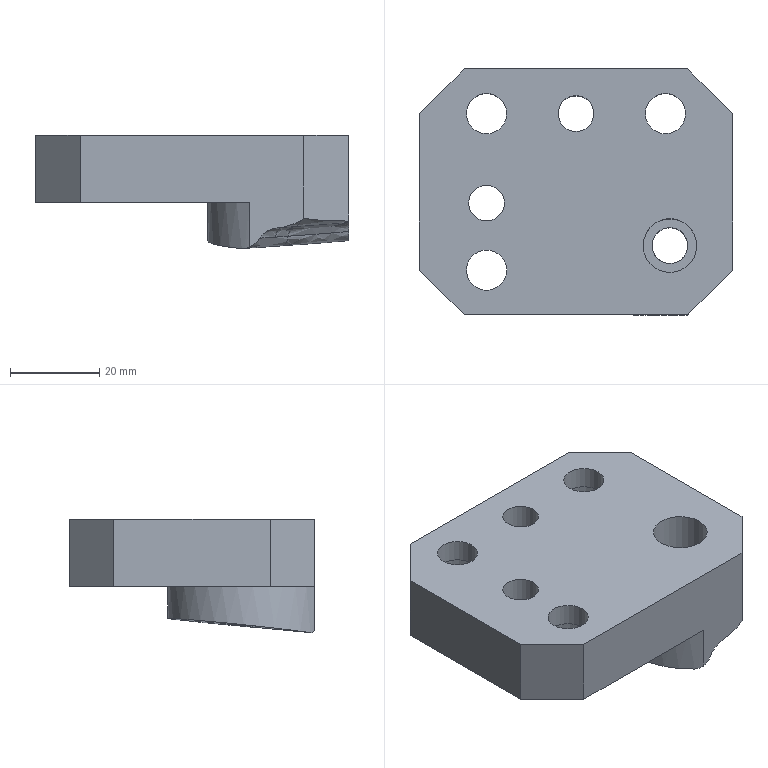Part | NX | features solid 2 | 1 solid | 36 faces | volume 52603 mm3 | plane 14 | spline 11 | cylinder 11 | commonest cylinder face diameters 8 x3 9 x3 14 x3 12 x1 35 x1